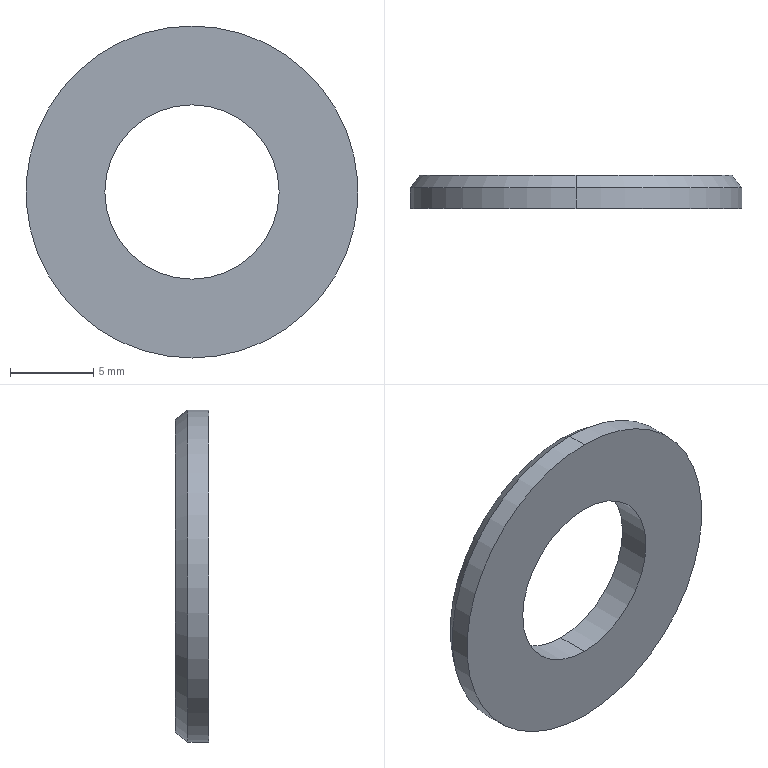Part | SolidWorks | features Chamfer 1, Extrusion 1 | 1 solid | 8 faces | box 20 x 2 x 20 mm | volume 441.839 mm3 | cylinder 4 | cone 2 | plane 2 | commonest cylinder face diameters 10.5 x2 20 x2
STEP:
#1=CARTESIAN_POINT('',(0.,2.,9.425));
#2=VERTEX_POINT('',#1);
#3=CARTESIAN_POINT('',(0.,2.,-9.425));
#4=VERTEX_POINT('',#3);
#5=CARTESIAN_POINT('',(0.,2.,0.));
#6=DIRECTION('',(0.,1.,0.));
#7=DIRECTION('',(0.,0.,1.));
#8=AXIS2_PLACEMENT_3D('',#5,#6,#7);
#9=CIRCLE('',#8,9.425);
#10=EDGE_CURVE('',#2,#4,#9,.T.);
#11=ORIENTED_EDGE('',*,*,#10,.F.);
#12=CARTESIAN_POINT('',(0.,1.25,10.));
#13=VERTEX_POINT('',#12);
#14=CARTESIAN_POINT('',(0.,2.,9.425));
#15=DIRECTION('',(0.,-0.7934,0.6088));
#16=VECTOR('',#15,1000.);
#17=LINE('',#14,#16);
#18=EDGE_CURVE('',#2,#13,#17,.T.);
#19=ORIENTED_EDGE('',*,*,#18,.T.);
#20=CARTESIAN_POINT('',(0.,1.25,-10.));
#21=VERTEX_POINT('',#20);
#22=CARTESIAN_POINT('',(0.,1.25,0.));
#23=DIRECTION('',(0.,-1.,0.));
#24=DIRECTION('',(0.,0.,1.));
#25=AXIS2_PLACEMENT_3D('',#22,#23,#24);
#26=CIRCLE('',#25,10.);
#27=EDGE_CURVE('',#21,#13,#26,.T.);
#28=ORIENTED_EDGE('',*,*,#27,.F.);
#29=CARTESIAN_POINT('',(0.,2.,-9.425));
#30=DIRECTION('',(0.,-0.7934,-0.6088));
#31=VECTOR('',#30,1000.);
#32=LINE('',#29,#31);
#33=EDGE_CURVE('',#4,#21,#32,.T.);
#34=ORIENTED_EDGE('',*,*,#33,.F.);
#35=EDGE_LOOP('',(#11,#19,#28,#34));
#36=FACE_OUTER_BOUND('',#35,.T.);
#37=CARTESIAN_POINT('',(0.,2.,0.));
#38=DIRECTION('',(0.,-1.,0.));
#39=DIRECTION('',(0.,0.,-1.));
#40=AXIS2_PLACEMENT_3D('',#37,#38,#39);
#41=CONICAL_SURFACE('',#40,9.425,0.6545);
#42=ADVANCED_FACE('',(#36),#41,.T.);
#43=CARTESIAN_POINT('',(0.,2.,-5.25));
#44=VERTEX_POINT('',#43);
#45=CARTESIAN_POINT('',(0.,2.,5.25));
#46=VERTEX_POINT('',#45);
#47=CARTESIAN_POINT('',(0.,2.,0.));
#48=DIRECTION('',(0.,1.,0.));
#49=DIRECTION('',(0.,0.,1.));
#50=AXIS2_PLACEMENT_3D('',#47,#48,#49);
#51=CIRCLE('',#50,5.25);
#52=EDGE_CURVE('',#44,#46,#51,.T.);
#53=ORIENTED_EDGE('',*,*,#52,.T.);
#54=CARTESIAN_POINT('',(0.,0.,5.25));
#55=VERTEX_POINT('',#54);
#56=CARTESIAN_POINT('',(0.,2.,5.25));
#57=DIRECTION('',(0.,-1.,0.));
#58=VECTOR('',#57,1000.);
#59=LINE('',#56,#58);
#60=EDGE_CURVE('',#46,#55,#59,.T.);
#61=ORIENTED_EDGE('',*,*,#60,.T.);
#62=CARTESIAN_POINT('',(0.,0.,-5.25));
#63=VERTEX_POINT('',#62);
#64=CARTESIAN_POINT('',(0.,0.,0.));
#65=DIRECTION('',(0.,1.,0.));
#66=DIRECTION('',(0.,0.,1.));
#67=AXIS2_PLACEMENT_3D('',#64,#65,#66);
#68=CIRCLE('',#67,5.25);
#69=EDGE_CURVE('',#63,#55,#68,.T.);
#70=ORIENTED_EDGE('',*,*,#69,.F.);
#71=CARTESIAN_POINT('',(0.,2.,-5.25));
#72=DIRECTION('',(0.,-1.,0.));
#73=VECTOR('',#72,1000.);
#74=LINE('',#71,#73);
#75=EDGE_CURVE('',#44,#63,#74,.T.);
#76=ORIENTED_EDGE('',*,*,#75,.F.);
#77=EDGE_LOOP('',(#53,#61,#70,#76));
#78=FACE_OUTER_BOUND('',#77,.T.);
#79=CARTESIAN_POINT('',(0.,2.,0.));
#80=DIRECTION('',(0.,-1.,0.));
#81=DIRECTION('',(0.,0.,-1.));
#82=AXIS2_PLACEMENT_3D('',#79,#80,#81);
#83=CYLINDRICAL_SURFACE('',#82,5.25);
#84=ADVANCED_FACE('',(#78),#83,.F.);
#85=ORIENTED_EDGE('',*,*,#27,.T.);
#86=CARTESIAN_POINT('',(0.,0.,10.));
#87=VERTEX_POINT('',#86);
#88=CARTESIAN_POINT('',(0.,2.,10.));
#89=DIRECTION('',(0.,-1.,0.));
#90=VECTOR('',#89,1000.);
#91=LINE('',#88,#90);
#92=EDGE_CURVE('',#13,#87,#91,.T.);
#93=ORIENTED_EDGE('',*,*,#92,.T.);
#94=CARTESIAN_POINT('',(0.,0.,-10.));
#95=VERTEX_POINT('',#94);
#96=CARTESIAN_POINT('',(0.,0.,0.));
#97=DIRECTION('',(0.,1.,0.));
#98=DIRECTION('',(0.,0.,1.));
#99=AXIS2_PLACEMENT_3D('',#96,#97,#98);
#100=CIRCLE('',#99,10.);
#101=EDGE_CURVE('',#87,#95,#100,.T.);
#102=ORIENTED_EDGE('',*,*,#101,.T.);
#103=CARTESIAN_POINT('',(0.,2.,-10.));
#104=DIRECTION('',(0.,-1.,0.));
#105=VECTOR('',#104,1000.);
#106=LINE('',#103,#105);
#107=EDGE_CURVE('',#21,#95,#106,.T.);
#108=ORIENTED_EDGE('',*,*,#107,.F.);
#109=EDGE_LOOP('',(#85,#93,#102,#108));
#110=FACE_OUTER_BOUND('',#109,.T.);
#111=CARTESIAN_POINT('',(0.,2.,0.));
#112=DIRECTION('',(0.,-1.,0.));
#113=DIRECTION('',(0.,0.,-1.));
#114=AXIS2_PLACEMENT_3D('',#111,#112,#113);
#115=CYLINDRICAL_SURFACE('',#114,10.);
#116=ADVANCED_FACE('',(#110),#115,.T.);
#117=CARTESIAN_POINT('',(0.,2.,0.));
#118=DIRECTION('',(0.,1.,0.));
#119=DIRECTION('',(0.,0.,1.));
#120=AXIS2_PLACEMENT_3D('',#117,#118,#119);
#121=CIRCLE('',#120,9.425);
#122=EDGE_CURVE('',#4,#2,#121,.T.);
#123=ORIENTED_EDGE('',*,*,#122,.T.);
#124=ORIENTED_EDGE('',*,*,#10,.T.);
#125=EDGE_LOOP('',(#123,#124));
#126=FACE_OUTER_BOUND('',#125,.T.);
#127=ORIENTED_EDGE('',*,*,#52,.F.);
#128=CARTESIAN_POINT('',(0.,2.,0.));
#129=DIRECTION('',(0.,1.,0.));
#130=DIRECTION('',(0.,0.,1.));
#131=AXIS2_PLACEMENT_3D('',#128,#129,#130);
#132=CIRCLE('',#131,5.25);
#133=EDGE_CURVE('',#46,#44,#132,.T.);
#134=ORIENTED_EDGE('',*,*,#133,.F.);
#135=EDGE_LOOP('',(#127,#134));
#136=FACE_BOUND('',#135,.T.);
#137=CARTESIAN_POINT('',(0.,2.,0.));
#138=DIRECTION('',(0.,1.,0.));
#139=DIRECTION('',(0.,0.,1.));
#140=AXIS2_PLACEMENT_3D('',#137,#138,#139);
#141=PLANE('',#140);
#142=ADVANCED_FACE('',(#126,#136),#141,.T.);
#143=CARTESIAN_POINT('',(0.,0.,0.));
#144=DIRECTION('',(0.,1.,0.));
#145=DIRECTION('',(0.,0.,1.));
#146=AXIS2_PLACEMENT_3D('',#143,#144,#145);
#147=CIRCLE('',#146,10.);
#148=EDGE_CURVE('',#95,#87,#147,.T.);
#149=ORIENTED_EDGE('',*,*,#148,.F.);
#150=ORIENTED_EDGE('',*,*,#101,.F.);
#151=EDGE_LOOP('',(#149,#150));
#152=FACE_OUTER_BOUND('',#151,.T.);
#153=ORIENTED_EDGE('',*,*,#69,.T.);
#154=CARTESIAN_POINT('',(0.,0.,0.));
#155=DIRECTION('',(0.,1.,0.));
#156=DIRECTION('',(0.,0.,1.));
#157=AXIS2_PLACEMENT_3D('',#154,#155,#156);
#158=CIRCLE('',#157,5.25);
#159=EDGE_CURVE('',#55,#63,#158,.T.);
#160=ORIENTED_EDGE('',*,*,#159,.T.);
#161=EDGE_LOOP('',(#153,#160));
#162=FACE_BOUND('',#161,.T.);
#163=CARTESIAN_POINT('',(0.,0.,0.));
#164=DIRECTION('',(0.,1.,0.));
#165=DIRECTION('',(0.,0.,1.));
#166=AXIS2_PLACEMENT_3D('',#163,#164,#165);
#167=PLANE('',#166);
#168=ADVANCED_FACE('',(#152,#162),#167,.F.);
#169=ORIENTED_EDGE('',*,*,#92,.F.);
#170=CARTESIAN_POINT('',(0.,1.25,0.));
#171=DIRECTION('',(0.,-1.,0.));
#172=DIRECTION('',(0.,0.,1.));
#173=AXIS2_PLACEMENT_3D('',#170,#171,#172);
#174=CIRCLE('',#173,10.);
#175=EDGE_CURVE('',#13,#21,#174,.T.);
#176=ORIENTED_EDGE('',*,*,#175,.T.);
#177=ORIENTED_EDGE('',*,*,#107,.T.);
#178=ORIENTED_EDGE('',*,*,#148,.T.);
#179=EDGE_LOOP('',(#169,#176,#177,#178));
#180=FACE_OUTER_BOUND('',#179,.T.);
#181=CARTESIAN_POINT('',(0.,2.,0.));
#182=DIRECTION('',(0.,-1.,0.));
#183=DIRECTION('',(0.,0.,-1.));
#184=AXIS2_PLACEMENT_3D('',#181,#182,#183);
#185=CYLINDRICAL_SURFACE('',#184,10.);
#186=ADVANCED_FACE('',(#180),#185,.T.);
#187=ORIENTED_EDGE('',*,*,#60,.F.);
#188=ORIENTED_EDGE('',*,*,#133,.T.);
#189=ORIENTED_EDGE('',*,*,#75,.T.);
#190=ORIENTED_EDGE('',*,*,#159,.F.);
#191=EDGE_LOOP('',(#187,#188,#189,#190));
#192=FACE_OUTER_BOUND('',#191,.T.);
#193=CARTESIAN_POINT('',(0.,2.,0.));
#194=DIRECTION('',(0.,-1.,0.));
#195=DIRECTION('',(0.,0.,-1.));
#196=AXIS2_PLACEMENT_3D('',#193,#194,#195);
#197=CYLINDRICAL_SURFACE('',#196,5.25);
#198=ADVANCED_FACE('',(#192),#197,.F.);
#199=ORIENTED_EDGE('',*,*,#18,.F.);
#200=ORIENTED_EDGE('',*,*,#122,.F.);
#201=ORIENTED_EDGE('',*,*,#33,.T.);
#202=ORIENTED_EDGE('',*,*,#175,.F.);
#203=EDGE_LOOP('',(#199,#200,#201,#202));
#204=FACE_OUTER_BOUND('',#203,.T.);
#205=CARTESIAN_POINT('',(0.,2.,0.));
#206=DIRECTION('',(0.,-1.,0.));
#207=DIRECTION('',(0.,0.,-1.));
#208=AXIS2_PLACEMENT_3D('',#205,#206,#207);
#209=CONICAL_SURFACE('',#208,9.425,0.6545);
#210=ADVANCED_FACE('',(#204),#209,.T.);
#211=CLOSED_SHELL('',(#42,#84,#116,#142,#168,#186,#198,#210));
#212=MANIFOLD_SOLID_BREP('',#211);
#213=CARTESIAN_POINT('',(0.,0.,0.));
#214=DIRECTION('',(0.,0.,1.));
#215=DIRECTION('',(1.,0.,0.));
#216=AXIS2_PLACEMENT_3D('',#213,#214,#215);
#217=(LENGTH_UNIT()NAMED_UNIT(*)SI_UNIT(.MILLI.,.METRE.));
#218=UNCERTAINTY_MEASURE_WITH_UNIT(LENGTH_MEASURE(0.00001),#217,'','');
#219=(NAMED_UNIT(*)PLANE_ANGLE_UNIT()SI_UNIT($,.RADIAN.));
#220=(NAMED_UNIT(*)SI_UNIT($,.STERADIAN.)SOLID_ANGLE_UNIT());
#221=(GEOMETRIC_REPRESENTATION_CONTEXT(3)GLOBAL_UNCERTAINTY_ASSIGNED_CONTEXT((#218))GLOBAL_UNIT_ASSIGNED_CONTEXT((#217,#219,#220))REPRESENTATION_CONTEXT('',''));
#222=ADVANCED_BREP_SHAPE_REPRESENTATION('',(#212,#216),#221);